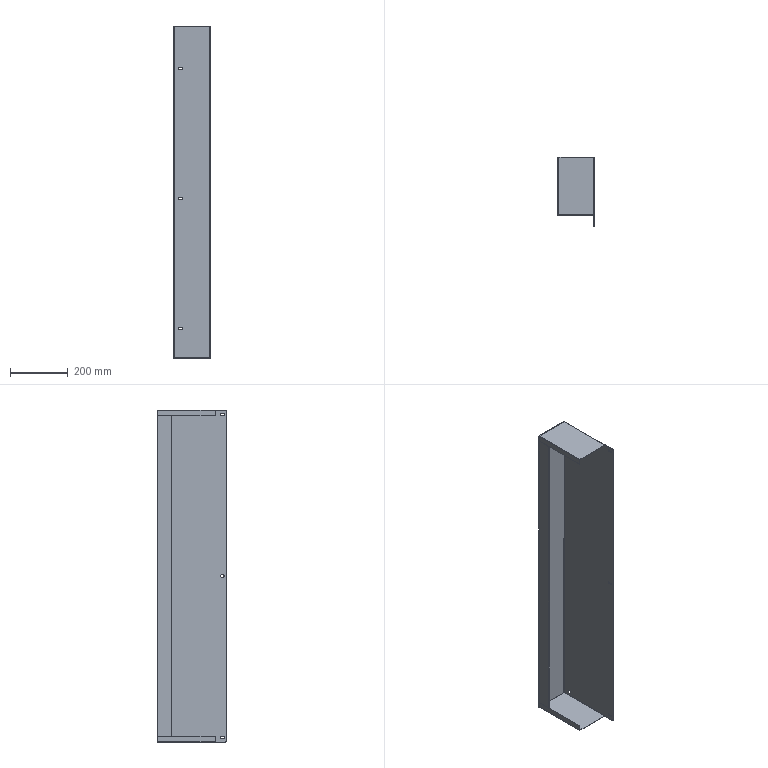Part | SolidWorks | features BaseBody 1 | 1 solid | 117 faces | box 125 x 240 x 1150 mm | volume 632507 mm3 | plane 84 | cylinder 29 | spline 4 | commonest cylinder face diameters 7 x15 1 x6 3.4 x6 10 x2